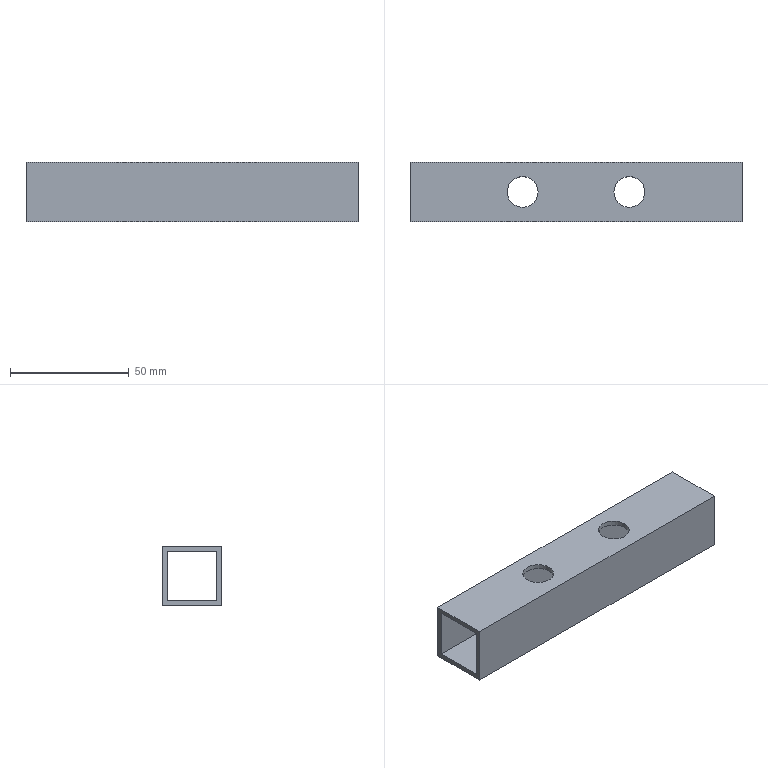Part | NX | features solid 2 | 1 solid | 14 faces | box 140 x 25 x 25 mm | volume 24698 mm3 | plane 10 | cylinder 4 | commonest cylinder face diameters 13 x4
STEP:
#1=CARTESIAN_POINT('',(226.,100.,10.));
#2=VERTEX_POINT('',#1);
#3=CARTESIAN_POINT('',(232.5,100.,10.));
#4=DIRECTION('',(0.,0.,-1.));
#5=DIRECTION('',(-1.,0.,0.));
#6=AXIS2_PLACEMENT_3D('',#3,#4,#5);
#7=CIRCLE('',#6,6.5);
#8=EDGE_CURVE('',#2,#2,#7,.T.);
#9=ORIENTED_EDGE('',*,*,#8,.F.);
#10=EDGE_LOOP('',(#9));
#11=FACE_BOUND('',#10,.T.);
#12=CARTESIAN_POINT('',(226.,100.,8.));
#13=VERTEX_POINT('',#12);
#14=CARTESIAN_POINT('',(232.5,100.,8.));
#15=DIRECTION('',(0.,0.,-1.));
#16=DIRECTION('',(-1.,0.,0.));
#17=AXIS2_PLACEMENT_3D('',#14,#15,#16);
#18=CIRCLE('',#17,6.5);
#19=EDGE_CURVE('',#13,#13,#18,.F.);
#20=ORIENTED_EDGE('',*,*,#19,.F.);
#21=EDGE_LOOP('',(#20));
#22=FACE_BOUND('',#21,.T.);
#23=CARTESIAN_POINT('',(232.5,100.,-25.));
#24=DIRECTION('',(0.,0.,1.));
#25=DIRECTION('',(1.,0.,0.));
#26=AXIS2_PLACEMENT_3D('',#23,#24,#25);
#27=CYLINDRICAL_SURFACE('',#26,6.5);
#28=ADVANCED_FACE('',(#11,#22),#27,.F.);
#29=CARTESIAN_POINT('',(271.,100.,10.));
#30=VERTEX_POINT('',#29);
#31=CARTESIAN_POINT('',(277.5,100.,10.));
#32=DIRECTION('',(0.,0.,-1.));
#33=DIRECTION('',(-1.,0.,0.));
#34=AXIS2_PLACEMENT_3D('',#31,#32,#33);
#35=CIRCLE('',#34,6.5);
#36=EDGE_CURVE('',#30,#30,#35,.F.);
#37=ORIENTED_EDGE('',*,*,#36,.T.);
#38=EDGE_LOOP('',(#37));
#39=FACE_BOUND('',#38,.T.);
#40=CARTESIAN_POINT('',(271.,100.,8.));
#41=VERTEX_POINT('',#40);
#42=CARTESIAN_POINT('',(277.5,100.,8.));
#43=DIRECTION('',(0.,0.,-1.));
#44=DIRECTION('',(-1.,0.,0.));
#45=AXIS2_PLACEMENT_3D('',#42,#43,#44);
#46=CIRCLE('',#45,6.5);
#47=EDGE_CURVE('',#41,#41,#46,.T.);
#48=ORIENTED_EDGE('',*,*,#47,.T.);
#49=EDGE_LOOP('',(#48));
#50=FACE_BOUND('',#49,.T.);
#51=CARTESIAN_POINT('',(277.5,100.,-14.));
#52=DIRECTION('',(0.,0.,1.));
#53=DIRECTION('',(1.,0.,0.));
#54=AXIS2_PLACEMENT_3D('',#51,#52,#53);
#55=CYLINDRICAL_SURFACE('',#54,6.5);
#56=ADVANCED_FACE('',(#39,#50),#55,.F.);
#57=CARTESIAN_POINT('',(325.,87.5,10.));
#58=VERTEX_POINT('',#57);
#59=CARTESIAN_POINT('',(325.,112.5,10.));
#60=VERTEX_POINT('',#59);
#61=CARTESIAN_POINT('',(325.,-135.,10.));
#62=DIRECTION('',(0.,1.,0.));
#63=VECTOR('',#62,1000.);
#64=LINE('',#61,#63);
#65=EDGE_CURVE('',#58,#60,#64,.T.);
#66=ORIENTED_EDGE('',*,*,#65,.F.);
#67=CARTESIAN_POINT('',(325.,87.5,-15.));
#68=VERTEX_POINT('',#67);
#69=CARTESIAN_POINT('',(325.,87.5,-15.));
#70=DIRECTION('',(0.,0.,1.));
#71=VECTOR('',#70,1000.);
#72=LINE('',#69,#71);
#73=EDGE_CURVE('',#58,#68,#72,.F.);
#74=ORIENTED_EDGE('',*,*,#73,.T.);
#75=CARTESIAN_POINT('',(325.,112.5,-15.));
#76=VERTEX_POINT('',#75);
#77=CARTESIAN_POINT('',(325.,-135.,-15.));
#78=DIRECTION('',(0.,1.,0.));
#79=VECTOR('',#78,1000.);
#80=LINE('',#77,#79);
#81=EDGE_CURVE('',#68,#76,#80,.T.);
#82=ORIENTED_EDGE('',*,*,#81,.T.);
#83=CARTESIAN_POINT('',(325.,112.5,-15.));
#84=DIRECTION('',(0.,0.,1.));
#85=VECTOR('',#84,1000.);
#86=LINE('',#83,#85);
#87=EDGE_CURVE('',#76,#60,#86,.T.);
#88=ORIENTED_EDGE('',*,*,#87,.T.);
#89=EDGE_LOOP('',(#66,#74,#82,#88));
#90=FACE_BOUND('',#89,.T.);
#91=CARTESIAN_POINT('',(325.,89.5,8.));
#92=VERTEX_POINT('',#91);
#93=CARTESIAN_POINT('',(325.,89.5,-13.));
#94=VERTEX_POINT('',#93);
#95=CARTESIAN_POINT('',(325.,89.5,-15.));
#96=DIRECTION('',(0.,0.,1.));
#97=VECTOR('',#96,1000.);
#98=LINE('',#95,#97);
#99=EDGE_CURVE('',#92,#94,#98,.F.);
#100=ORIENTED_EDGE('',*,*,#99,.F.);
#101=CARTESIAN_POINT('',(325.,110.5,8.));
#102=VERTEX_POINT('',#101);
#103=CARTESIAN_POINT('',(325.,-135.,8.));
#104=DIRECTION('',(0.,1.,0.));
#105=VECTOR('',#104,1000.);
#106=LINE('',#103,#105);
#107=EDGE_CURVE('',#92,#102,#106,.T.);
#108=ORIENTED_EDGE('',*,*,#107,.T.);
#109=CARTESIAN_POINT('',(325.,110.5,-13.));
#110=VERTEX_POINT('',#109);
#111=CARTESIAN_POINT('',(325.,110.5,-15.));
#112=DIRECTION('',(0.,0.,1.));
#113=VECTOR('',#112,1000.);
#114=LINE('',#111,#113);
#115=EDGE_CURVE('',#110,#102,#114,.T.);
#116=ORIENTED_EDGE('',*,*,#115,.F.);
#117=CARTESIAN_POINT('',(325.,-135.,-13.));
#118=DIRECTION('',(0.,1.,0.));
#119=VECTOR('',#118,1000.);
#120=LINE('',#117,#119);
#121=EDGE_CURVE('',#94,#110,#120,.T.);
#122=ORIENTED_EDGE('',*,*,#121,.F.);
#123=EDGE_LOOP('',(#100,#108,#116,#122));
#124=FACE_BOUND('',#123,.T.);
#125=CARTESIAN_POINT('',(325.,-135.,-15.));
#126=DIRECTION('',(1.,0.,0.));
#127=DIRECTION('',(0.,0.,1.));
#128=AXIS2_PLACEMENT_3D('',#125,#126,#127);
#129=PLANE('',#128);
#130=ADVANCED_FACE('',(#90,#124),#129,.T.);
#131=CARTESIAN_POINT('',(271.,100.,-15.));
#132=VERTEX_POINT('',#131);
#133=CARTESIAN_POINT('',(277.5,100.,-15.));
#134=DIRECTION('',(0.,0.,-1.));
#135=DIRECTION('',(-1.,0.,0.));
#136=AXIS2_PLACEMENT_3D('',#133,#134,#135);
#137=CIRCLE('',#136,6.5);
#138=EDGE_CURVE('',#132,#132,#137,.F.);
#139=ORIENTED_EDGE('',*,*,#138,.T.);
#140=EDGE_LOOP('',(#139));
#141=FACE_BOUND('',#140,.T.);
#142=CARTESIAN_POINT('',(226.,100.,-15.));
#143=VERTEX_POINT('',#142);
#144=CARTESIAN_POINT('',(232.5,100.,-15.));
#145=DIRECTION('',(0.,0.,-1.));
#146=DIRECTION('',(-1.,0.,0.));
#147=AXIS2_PLACEMENT_3D('',#144,#145,#146);
#148=CIRCLE('',#147,6.5);
#149=EDGE_CURVE('',#143,#143,#148,.T.);
#150=ORIENTED_EDGE('',*,*,#149,.F.);
#151=EDGE_LOOP('',(#150));
#152=FACE_BOUND('',#151,.T.);
#153=ORIENTED_EDGE('',*,*,#81,.F.);
#154=CARTESIAN_POINT('',(185.,87.5,-15.));
#155=VERTEX_POINT('',#154);
#156=CARTESIAN_POINT('',(292.5,87.5,-15.));
#157=DIRECTION('',(1.,0.,0.));
#158=VECTOR('',#157,1000.);
#159=LINE('',#156,#158);
#160=EDGE_CURVE('',#68,#155,#159,.F.);
#161=ORIENTED_EDGE('',*,*,#160,.T.);
#162=CARTESIAN_POINT('',(185.,112.5,-15.));
#163=VERTEX_POINT('',#162);
#164=CARTESIAN_POINT('',(185.,85.,-15.));
#165=DIRECTION('',(0.,-1.,0.));
#166=VECTOR('',#165,1000.);
#167=LINE('',#164,#166);
#168=EDGE_CURVE('',#155,#163,#167,.F.);
#169=ORIENTED_EDGE('',*,*,#168,.T.);
#170=CARTESIAN_POINT('',(292.5,112.5,-15.));
#171=DIRECTION('',(-1.,0.,0.));
#172=VECTOR('',#171,1000.);
#173=LINE('',#170,#172);
#174=EDGE_CURVE('',#76,#163,#173,.T.);
#175=ORIENTED_EDGE('',*,*,#174,.F.);
#176=EDGE_LOOP('',(#153,#161,#169,#175));
#177=FACE_BOUND('',#176,.T.);
#178=CARTESIAN_POINT('',(292.5,85.,-15.));
#179=DIRECTION('',(0.,0.,-1.));
#180=DIRECTION('',(-1.,0.,0.));
#181=AXIS2_PLACEMENT_3D('',#178,#179,#180);
#182=PLANE('',#181);
#183=ADVANCED_FACE('',(#141,#152,#177),#182,.T.);
#184=ORIENTED_EDGE('',*,*,#36,.F.);
#185=EDGE_LOOP('',(#184));
#186=FACE_BOUND('',#185,.T.);
#187=ORIENTED_EDGE('',*,*,#8,.T.);
#188=EDGE_LOOP('',(#187));
#189=FACE_BOUND('',#188,.T.);
#190=CARTESIAN_POINT('',(185.,87.5,10.));
#191=VERTEX_POINT('',#190);
#192=CARTESIAN_POINT('',(292.5,87.5,10.));
#193=DIRECTION('',(1.,0.,0.));
#194=VECTOR('',#193,1000.);
#195=LINE('',#192,#194);
#196=EDGE_CURVE('',#58,#191,#195,.F.);
#197=ORIENTED_EDGE('',*,*,#196,.F.);
#198=ORIENTED_EDGE('',*,*,#65,.T.);
#199=CARTESIAN_POINT('',(185.,112.5,10.));
#200=VERTEX_POINT('',#199);
#201=CARTESIAN_POINT('',(292.5,112.5,10.));
#202=DIRECTION('',(-1.,0.,0.));
#203=VECTOR('',#202,1000.);
#204=LINE('',#201,#203);
#205=EDGE_CURVE('',#60,#200,#204,.T.);
#206=ORIENTED_EDGE('',*,*,#205,.T.);
#207=CARTESIAN_POINT('',(185.,85.,10.));
#208=DIRECTION('',(0.,-1.,0.));
#209=VECTOR('',#208,1000.);
#210=LINE('',#207,#209);
#211=EDGE_CURVE('',#191,#200,#210,.F.);
#212=ORIENTED_EDGE('',*,*,#211,.F.);
#213=EDGE_LOOP('',(#197,#198,#206,#212));
#214=FACE_BOUND('',#213,.T.);
#215=CARTESIAN_POINT('',(292.5,85.,10.));
#216=DIRECTION('',(0.,0.,-1.));
#217=DIRECTION('',(-1.,0.,0.));
#218=AXIS2_PLACEMENT_3D('',#215,#216,#217);
#219=PLANE('',#218);
#220=ADVANCED_FACE('',(#186,#189,#214),#219,.F.);
#221=CARTESIAN_POINT('',(185.,89.5,-13.));
#222=VERTEX_POINT('',#221);
#223=CARTESIAN_POINT('',(185.,89.5,8.));
#224=VERTEX_POINT('',#223);
#225=CARTESIAN_POINT('',(185.,89.5,-15.));
#226=DIRECTION('',(0.,0.,-1.));
#227=VECTOR('',#226,1000.);
#228=LINE('',#225,#227);
#229=EDGE_CURVE('',#222,#224,#228,.F.);
#230=ORIENTED_EDGE('',*,*,#229,.F.);
#231=CARTESIAN_POINT('',(185.,110.5,-13.));
#232=VERTEX_POINT('',#231);
#233=CARTESIAN_POINT('',(185.,-135.,-13.));
#234=DIRECTION('',(0.,1.,0.));
#235=VECTOR('',#234,1000.);
#236=LINE('',#233,#235);
#237=EDGE_CURVE('',#232,#222,#236,.F.);
#238=ORIENTED_EDGE('',*,*,#237,.F.);
#239=CARTESIAN_POINT('',(185.,110.5,8.));
#240=VERTEX_POINT('',#239);
#241=CARTESIAN_POINT('',(185.,110.5,-15.));
#242=DIRECTION('',(0.,0.,1.));
#243=VECTOR('',#242,1000.);
#244=LINE('',#241,#243);
#245=EDGE_CURVE('',#240,#232,#244,.F.);
#246=ORIENTED_EDGE('',*,*,#245,.F.);
#247=CARTESIAN_POINT('',(185.,-135.,8.));
#248=DIRECTION('',(0.,1.,0.));
#249=VECTOR('',#248,1000.);
#250=LINE('',#247,#249);
#251=EDGE_CURVE('',#240,#224,#250,.F.);
#252=ORIENTED_EDGE('',*,*,#251,.T.);
#253=EDGE_LOOP('',(#230,#238,#246,#252));
#254=FACE_BOUND('',#253,.T.);
#255=ORIENTED_EDGE('',*,*,#168,.F.);
#256=CARTESIAN_POINT('',(185.,87.5,-15.));
#257=DIRECTION('',(0.,0.,1.));
#258=VECTOR('',#257,1000.);
#259=LINE('',#256,#258);
#260=EDGE_CURVE('',#155,#191,#259,.T.);
#261=ORIENTED_EDGE('',*,*,#260,.T.);
#262=ORIENTED_EDGE('',*,*,#211,.T.);
#263=CARTESIAN_POINT('',(185.,112.5,-15.));
#264=DIRECTION('',(0.,0.,-1.));
#265=VECTOR('',#264,1000.);
#266=LINE('',#263,#265);
#267=EDGE_CURVE('',#163,#200,#266,.F.);
#268=ORIENTED_EDGE('',*,*,#267,.F.);
#269=EDGE_LOOP('',(#255,#261,#262,#268));
#270=FACE_BOUND('',#269,.T.);
#271=CARTESIAN_POINT('',(185.,-135.,-15.));
#272=DIRECTION('',(1.,0.,0.));
#273=DIRECTION('',(0.,0.,1.));
#274=AXIS2_PLACEMENT_3D('',#271,#272,#273);
#275=PLANE('',#274);
#276=ADVANCED_FACE('',(#254,#270),#275,.F.);
#277=ORIENTED_EDGE('',*,*,#260,.F.);
#278=ORIENTED_EDGE('',*,*,#160,.F.);
#279=ORIENTED_EDGE('',*,*,#73,.F.);
#280=ORIENTED_EDGE('',*,*,#196,.T.);
#281=EDGE_LOOP('',(#277,#278,#279,#280));
#282=FACE_BOUND('',#281,.T.);
#283=CARTESIAN_POINT('',(292.5,87.5,-15.));
#284=DIRECTION('',(0.,-1.,0.));
#285=DIRECTION('',(-1.,0.,0.));
#286=AXIS2_PLACEMENT_3D('',#283,#284,#285);
#287=PLANE('',#286);
#288=ADVANCED_FACE('',(#282),#287,.T.);
#289=ORIENTED_EDGE('',*,*,#174,.T.);
#290=ORIENTED_EDGE('',*,*,#267,.T.);
#291=ORIENTED_EDGE('',*,*,#205,.F.);
#292=ORIENTED_EDGE('',*,*,#87,.F.);
#293=EDGE_LOOP('',(#289,#290,#291,#292));
#294=FACE_BOUND('',#293,.T.);
#295=CARTESIAN_POINT('',(292.5,112.5,-15.));
#296=DIRECTION('',(0.,-1.,0.));
#297=DIRECTION('',(-1.,0.,0.));
#298=AXIS2_PLACEMENT_3D('',#295,#296,#297);
#299=PLANE('',#298);
#300=ADVANCED_FACE('',(#294),#299,.F.);
#301=CARTESIAN_POINT('',(226.,100.,-13.));
#302=VERTEX_POINT('',#301);
#303=CARTESIAN_POINT('',(232.5,100.,-13.));
#304=DIRECTION('',(0.,0.,-1.));
#305=DIRECTION('',(-1.,0.,0.));
#306=AXIS2_PLACEMENT_3D('',#303,#304,#305);
#307=CIRCLE('',#306,6.5);
#308=EDGE_CURVE('',#302,#302,#307,.F.);
#309=ORIENTED_EDGE('',*,*,#308,.T.);
#310=EDGE_LOOP('',(#309));
#311=FACE_BOUND('',#310,.T.);
#312=ORIENTED_EDGE('',*,*,#149,.T.);
#313=EDGE_LOOP('',(#312));
#314=FACE_BOUND('',#313,.T.);
#315=CARTESIAN_POINT('',(232.5,100.,-25.));
#316=DIRECTION('',(0.,0.,1.));
#317=DIRECTION('',(1.,0.,0.));
#318=AXIS2_PLACEMENT_3D('',#315,#316,#317);
#319=CYLINDRICAL_SURFACE('',#318,6.5);
#320=ADVANCED_FACE('',(#311,#314),#319,.F.);
#321=CARTESIAN_POINT('',(271.,100.,-13.));
#322=VERTEX_POINT('',#321);
#323=CARTESIAN_POINT('',(277.5,100.,-13.));
#324=DIRECTION('',(0.,0.,-1.));
#325=DIRECTION('',(-1.,0.,0.));
#326=AXIS2_PLACEMENT_3D('',#323,#324,#325);
#327=CIRCLE('',#326,6.5);
#328=EDGE_CURVE('',#322,#322,#327,.T.);
#329=ORIENTED_EDGE('',*,*,#328,.F.);
#330=EDGE_LOOP('',(#329));
#331=FACE_BOUND('',#330,.T.);
#332=ORIENTED_EDGE('',*,*,#138,.F.);
#333=EDGE_LOOP('',(#332));
#334=FACE_BOUND('',#333,.T.);
#335=CARTESIAN_POINT('',(277.5,100.,-14.));
#336=DIRECTION('',(0.,0.,1.));
#337=DIRECTION('',(1.,0.,0.));
#338=AXIS2_PLACEMENT_3D('',#335,#336,#337);
#339=CYLINDRICAL_SURFACE('',#338,6.5);
#340=ADVANCED_FACE('',(#331,#334),#339,.F.);
#341=ORIENTED_EDGE('',*,*,#121,.T.);
#342=CARTESIAN_POINT('',(292.5,110.5,-13.));
#343=DIRECTION('',(-1.,0.,0.));
#344=VECTOR('',#343,1000.);
#345=LINE('',#342,#344);
#346=EDGE_CURVE('',#110,#232,#345,.T.);
#347=ORIENTED_EDGE('',*,*,#346,.T.);
#348=ORIENTED_EDGE('',*,*,#237,.T.);
#349=CARTESIAN_POINT('',(292.5,89.5,-13.));
#350=DIRECTION('',(1.,0.,0.));
#351=VECTOR('',#350,1000.);
#352=LINE('',#349,#351);
#353=EDGE_CURVE('',#94,#222,#352,.F.);
#354=ORIENTED_EDGE('',*,*,#353,.F.);
#355=EDGE_LOOP('',(#341,#347,#348,#354));
#356=FACE_BOUND('',#355,.T.);
#357=ORIENTED_EDGE('',*,*,#328,.T.);
#358=EDGE_LOOP('',(#357));
#359=FACE_BOUND('',#358,.T.);
#360=ORIENTED_EDGE('',*,*,#308,.F.);
#361=EDGE_LOOP('',(#360));
#362=FACE_BOUND('',#361,.T.);
#363=CARTESIAN_POINT('',(292.5,85.,-13.));
#364=DIRECTION('',(0.,0.,-1.));
#365=DIRECTION('',(-1.,0.,0.));
#366=AXIS2_PLACEMENT_3D('',#363,#364,#365);
#367=PLANE('',#366);
#368=ADVANCED_FACE('',(#356,#359,#362),#367,.F.);
#369=CARTESIAN_POINT('',(292.5,89.5,8.));
#370=DIRECTION('',(1.,0.,0.));
#371=VECTOR('',#370,1000.);
#372=LINE('',#369,#371);
#373=EDGE_CURVE('',#92,#224,#372,.F.);
#374=ORIENTED_EDGE('',*,*,#373,.T.);
#375=ORIENTED_EDGE('',*,*,#251,.F.);
#376=CARTESIAN_POINT('',(292.5,110.5,8.));
#377=DIRECTION('',(-1.,0.,0.));
#378=VECTOR('',#377,1000.);
#379=LINE('',#376,#378);
#380=EDGE_CURVE('',#102,#240,#379,.T.);
#381=ORIENTED_EDGE('',*,*,#380,.F.);
#382=ORIENTED_EDGE('',*,*,#107,.F.);
#383=EDGE_LOOP('',(#374,#375,#381,#382));
#384=FACE_BOUND('',#383,.T.);
#385=ORIENTED_EDGE('',*,*,#47,.F.);
#386=EDGE_LOOP('',(#385));
#387=FACE_BOUND('',#386,.T.);
#388=ORIENTED_EDGE('',*,*,#19,.T.);
#389=EDGE_LOOP('',(#388));
#390=FACE_BOUND('',#389,.T.);
#391=CARTESIAN_POINT('',(292.5,85.,8.));
#392=DIRECTION('',(0.,0.,-1.));
#393=DIRECTION('',(-1.,0.,0.));
#394=AXIS2_PLACEMENT_3D('',#391,#392,#393);
#395=PLANE('',#394);
#396=ADVANCED_FACE('',(#384,#387,#390),#395,.T.);
#397=ORIENTED_EDGE('',*,*,#353,.T.);
#398=ORIENTED_EDGE('',*,*,#229,.T.);
#399=ORIENTED_EDGE('',*,*,#373,.F.);
#400=ORIENTED_EDGE('',*,*,#99,.T.);
#401=EDGE_LOOP('',(#397,#398,#399,#400));
#402=FACE_BOUND('',#401,.T.);
#403=CARTESIAN_POINT('',(292.5,89.5,-15.));
#404=DIRECTION('',(0.,-1.,0.));
#405=DIRECTION('',(-1.,0.,0.));
#406=AXIS2_PLACEMENT_3D('',#403,#404,#405);
#407=PLANE('',#406);
#408=ADVANCED_FACE('',(#402),#407,.F.);
#409=ORIENTED_EDGE('',*,*,#346,.F.);
#410=ORIENTED_EDGE('',*,*,#115,.T.);
#411=ORIENTED_EDGE('',*,*,#380,.T.);
#412=ORIENTED_EDGE('',*,*,#245,.T.);
#413=EDGE_LOOP('',(#409,#410,#411,#412));
#414=FACE_BOUND('',#413,.T.);
#415=CARTESIAN_POINT('',(292.5,110.5,-15.));
#416=DIRECTION('',(0.,-1.,0.));
#417=DIRECTION('',(-1.,0.,0.));
#418=AXIS2_PLACEMENT_3D('',#415,#416,#417);
#419=PLANE('',#418);
#420=ADVANCED_FACE('',(#414),#419,.T.);
#421=CLOSED_SHELL('',(#28,#56,#130,#183,#220,#276,#288,#300,#320,#340,#368,#396,#408,#420));
#422=MANIFOLD_SOLID_BREP('',#421);
#423=(LENGTH_UNIT()NAMED_UNIT(*)SI_UNIT(.MILLI.,.METRE.));
#424=UNCERTAINTY_MEASURE_WITH_UNIT(LENGTH_MEASURE(0.00001),#423,'','');
#425=(NAMED_UNIT(*)PLANE_ANGLE_UNIT()SI_UNIT($,.RADIAN.));
#426=(NAMED_UNIT(*)SI_UNIT($,.STERADIAN.)SOLID_ANGLE_UNIT());
#427=(GEOMETRIC_REPRESENTATION_CONTEXT(3)GLOBAL_UNCERTAINTY_ASSIGNED_CONTEXT((#424))GLOBAL_UNIT_ASSIGNED_CONTEXT((#423,#425,#426))REPRESENTATION_CONTEXT('',''));
#428=ADVANCED_BREP_SHAPE_REPRESENTATION('',(#422),#427);